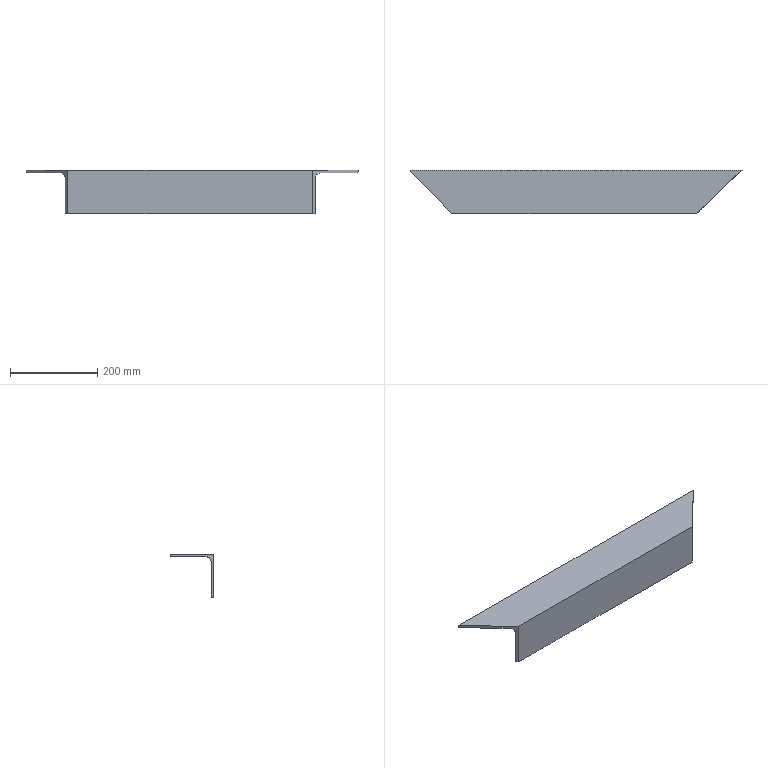Part | SolidWorks | features Extrusion 1, ICE 1 | 1 solid | 11 faces | box 761.728 x 100 x 100 mm | volume 732885 mm3 | plane 8 | cylinder 3 | commonest cylinder face diameters 5.4 x2 24 x1
STEP:
#1=CARTESIAN_POINT('',(-821.429,-32.,44.));
#2=VERTEX_POINT('',#1);
#3=CARTESIAN_POINT('',(-809.931,-44.,32.));
#4=VERTEX_POINT('',#3);
#5=CARTESIAN_POINT('',(-821.429,-32.,44.));
#6=CARTESIAN_POINT('',(-814.694,-39.029,44.));
#7=CARTESIAN_POINT('',(-809.931,-44.,39.029));
#8=CARTESIAN_POINT('',(-809.931,-44.,32.));
#9=(BOUNDED_CURVE()B_SPLINE_CURVE(3,(#5,#6,#7,#8),.UNSPECIFIED.,.F.,.F.)B_SPLINE_CURVE_WITH_KNOTS((4,4),(1.571,3.142),.UNSPECIFIED.)CURVE()GEOMETRIC_REPRESENTATION_ITEM()RATIONAL_B_SPLINE_CURVE((1.,0.8047,0.8047,1.))REPRESENTATION_ITEM(''));
#10=EDGE_CURVE('',#2,#4,#9,.T.);
#11=ORIENTED_EDGE('',*,*,#10,.F.);
#12=CARTESIAN_POINT('',(-223.851,-32.,44.));
#13=VERTEX_POINT('',#12);
#14=CARTESIAN_POINT('',(900.,-32.,44.));
#15=DIRECTION('',(-1.,0.,0.));
#16=VECTOR('',#15,1000.);
#17=LINE('',#14,#16);
#18=EDGE_CURVE('',#13,#2,#17,.T.);
#19=ORIENTED_EDGE('',*,*,#18,.F.);
#20=CARTESIAN_POINT('',(-236.375,-44.,32.));
#21=VERTEX_POINT('',#20);
#22=CARTESIAN_POINT('',(-236.375,-44.,32.));
#23=CARTESIAN_POINT('',(-236.375,-44.,39.029));
#24=CARTESIAN_POINT('',(-231.187,-39.029,44.));
#25=CARTESIAN_POINT('',(-223.851,-32.,44.));
#26=(BOUNDED_CURVE()B_SPLINE_CURVE(3,(#22,#23,#24,#25),.UNSPECIFIED.,.F.,.F.)B_SPLINE_CURVE_WITH_KNOTS((4,4),(0.,1.571),.UNSPECIFIED.)CURVE()GEOMETRIC_REPRESENTATION_ITEM()RATIONAL_B_SPLINE_CURVE((1.,0.8047,0.8047,1.))REPRESENTATION_ITEM(''));
#27=EDGE_CURVE('',#21,#13,#26,.T.);
#28=ORIENTED_EDGE('',*,*,#27,.F.);
#29=CARTESIAN_POINT('',(900.,-44.,32.));
#30=DIRECTION('',(-1.,0.,0.));
#31=VECTOR('',#30,1000.);
#32=LINE('',#29,#31);
#33=EDGE_CURVE('',#21,#4,#32,.T.);
#34=ORIENTED_EDGE('',*,*,#33,.T.);
#35=EDGE_LOOP('',(#11,#19,#28,#34));
#36=FACE_OUTER_BOUND('',#35,.T.);
#37=CARTESIAN_POINT('',(900.,-32.,32.));
#38=DIRECTION('',(-1.,0.,0.));
#39=DIRECTION('',(0.,0.,1.));
#40=AXIS2_PLACEMENT_3D('',#37,#38,#39);
#41=CYLINDRICAL_SURFACE('',#40,12.);
#42=ADVANCED_FACE('',(#36),#41,.F.);
#43=CARTESIAN_POINT('',(-897.413,47.3,44.));
#44=VERTEX_POINT('',#43);
#45=CARTESIAN_POINT('',(-37.074,-850.587,44.));
#46=DIRECTION('',(0.6918,-0.722,0.));
#47=VECTOR('',#46,1000.);
#48=LINE('',#45,#47);
#49=EDGE_CURVE('',#44,#2,#48,.T.);
#50=ORIENTED_EDGE('',*,*,#49,.F.);
#51=CARTESIAN_POINT('',(-141.09,47.3,44.));
#52=VERTEX_POINT('',#51);
#53=CARTESIAN_POINT('',(900.,47.3,44.));
#54=DIRECTION('',(-1.,0.,0.));
#55=VECTOR('',#54,1000.);
#56=LINE('',#53,#55);
#57=EDGE_CURVE('',#52,#44,#56,.T.);
#58=ORIENTED_EDGE('',*,*,#57,.F.);
#59=CARTESIAN_POINT('',(401.678,567.371,44.));
#60=DIRECTION('',(0.722,0.6918,0.));
#61=VECTOR('',#60,1000.);
#62=LINE('',#59,#61);
#63=EDGE_CURVE('',#13,#52,#62,.T.);
#64=ORIENTED_EDGE('',*,*,#63,.F.);
#65=ORIENTED_EDGE('',*,*,#18,.T.);
#66=EDGE_LOOP('',(#50,#58,#64,#65));
#67=FACE_OUTER_BOUND('',#66,.T.);
#68=CARTESIAN_POINT('',(900.,47.3,44.));
#69=DIRECTION('',(0.,0.,1.));
#70=DIRECTION('',(0.,-1.,0.));
#71=AXIS2_PLACEMENT_3D('',#68,#69,#70);
#72=PLANE('',#71);
#73=ADVANCED_FACE('',(#67),#72,.F.);
#74=CARTESIAN_POINT('',(-900.,50.,46.7));
#75=VERTEX_POINT('',#74);
#76=CARTESIAN_POINT('',(-900.,50.,46.7));
#77=CARTESIAN_POINT('',(-900.,50.,45.118));
#78=CARTESIAN_POINT('',(-898.928,48.882,44.));
#79=CARTESIAN_POINT('',(-897.413,47.3,44.));
#80=(BOUNDED_CURVE()B_SPLINE_CURVE(3,(#76,#77,#78,#79),.UNSPECIFIED.,.F.,.F.)B_SPLINE_CURVE_WITH_KNOTS((4,4),(0.,1.571),.UNSPECIFIED.)CURVE()GEOMETRIC_REPRESENTATION_ITEM()RATIONAL_B_SPLINE_CURVE((1.,0.8047,0.8047,1.))REPRESENTATION_ITEM(''));
#81=EDGE_CURVE('',#75,#44,#80,.T.);
#82=ORIENTED_EDGE('',*,*,#81,.F.);
#83=CARTESIAN_POINT('',(-138.272,50.,46.7));
#84=VERTEX_POINT('',#83);
#85=CARTESIAN_POINT('',(900.,50.,46.7));
#86=DIRECTION('',(-1.,0.,0.));
#87=VECTOR('',#86,1000.);
#88=LINE('',#85,#87);
#89=EDGE_CURVE('',#84,#75,#88,.T.);
#90=ORIENTED_EDGE('',*,*,#89,.F.);
#91=CARTESIAN_POINT('',(-141.09,47.3,44.));
#92=CARTESIAN_POINT('',(-139.44,48.882,44.));
#93=CARTESIAN_POINT('',(-138.272,50.,45.118));
#94=CARTESIAN_POINT('',(-138.272,50.,46.7));
#95=(BOUNDED_CURVE()B_SPLINE_CURVE(3,(#91,#92,#93,#94),.UNSPECIFIED.,.F.,.F.)B_SPLINE_CURVE_WITH_KNOTS((4,4),(1.571,3.142),.UNSPECIFIED.)CURVE()GEOMETRIC_REPRESENTATION_ITEM()RATIONAL_B_SPLINE_CURVE((1.,0.8047,0.8047,1.))REPRESENTATION_ITEM(''));
#96=EDGE_CURVE('',#52,#84,#95,.T.);
#97=ORIENTED_EDGE('',*,*,#96,.F.);
#98=ORIENTED_EDGE('',*,*,#57,.T.);
#99=EDGE_LOOP('',(#82,#90,#97,#98));
#100=FACE_OUTER_BOUND('',#99,.T.);
#101=CARTESIAN_POINT('',(900.,47.3,46.7));
#102=DIRECTION('',(-1.,0.,0.));
#103=DIRECTION('',(0.,0.,1.));
#104=AXIS2_PLACEMENT_3D('',#101,#102,#103);
#105=CYLINDRICAL_SURFACE('',#104,2.7);
#106=ADVANCED_FACE('',(#100),#105,.T.);
#107=CARTESIAN_POINT('',(-138.272,50.,50.));
#108=VERTEX_POINT('',#107);
#109=CARTESIAN_POINT('',(-138.272,50.,-50.));
#110=DIRECTION('',(0.,0.,1.));
#111=VECTOR('',#110,1000.);
#112=LINE('',#109,#111);
#113=EDGE_CURVE('',#84,#108,#112,.T.);
#114=ORIENTED_EDGE('',*,*,#113,.F.);
#115=ORIENTED_EDGE('',*,*,#89,.T.);
#116=CARTESIAN_POINT('',(-900.,50.,50.));
#117=VERTEX_POINT('',#116);
#118=CARTESIAN_POINT('',(-900.,50.,50.));
#119=DIRECTION('',(0.,0.,1.));
#120=VECTOR('',#119,1000.);
#121=LINE('',#118,#120);
#122=EDGE_CURVE('',#75,#117,#121,.T.);
#123=ORIENTED_EDGE('',*,*,#122,.T.);
#124=CARTESIAN_POINT('',(900.,50.,50.));
#125=DIRECTION('',(-1.,0.,0.));
#126=VECTOR('',#125,1000.);
#127=LINE('',#124,#126);
#128=EDGE_CURVE('',#108,#117,#127,.T.);
#129=ORIENTED_EDGE('',*,*,#128,.F.);
#130=EDGE_LOOP('',(#114,#115,#123,#129));
#131=FACE_OUTER_BOUND('',#130,.T.);
#132=CARTESIAN_POINT('',(900.,50.,50.));
#133=DIRECTION('',(0.,-1.,0.));
#134=DIRECTION('',(0.,0.,-1.));
#135=AXIS2_PLACEMENT_3D('',#132,#133,#134);
#136=PLANE('',#135);
#137=ADVANCED_FACE('',(#131),#136,.F.);
#138=CARTESIAN_POINT('',(-804.182,-50.,50.));
#139=VERTEX_POINT('',#138);
#140=CARTESIAN_POINT('',(-900.,50.,50.));
#141=DIRECTION('',(0.6918,-0.722,0.));
#142=VECTOR('',#141,1000.);
#143=LINE('',#140,#142);
#144=EDGE_CURVE('',#117,#139,#143,.T.);
#145=ORIENTED_EDGE('',*,*,#144,.T.);
#146=CARTESIAN_POINT('',(-242.637,-50.,50.));
#147=VERTEX_POINT('',#146);
#148=CARTESIAN_POINT('',(900.,-50.,50.));
#149=DIRECTION('',(-1.,0.,0.));
#150=VECTOR('',#149,1000.);
#151=LINE('',#148,#150);
#152=EDGE_CURVE('',#147,#139,#151,.T.);
#153=ORIENTED_EDGE('',*,*,#152,.F.);
#154=CARTESIAN_POINT('',(-535.396,-330.517,50.));
#155=DIRECTION('',(0.722,0.6918,0.));
#156=VECTOR('',#155,1000.);
#157=LINE('',#154,#156);
#158=EDGE_CURVE('',#147,#108,#157,.T.);
#159=ORIENTED_EDGE('',*,*,#158,.T.);
#160=ORIENTED_EDGE('',*,*,#128,.T.);
#161=EDGE_LOOP('',(#145,#153,#159,#160));
#162=FACE_OUTER_BOUND('',#161,.T.);
#163=CARTESIAN_POINT('',(900.,-50.,50.));
#164=DIRECTION('',(0.,0.,-1.));
#165=DIRECTION('',(0.,1.,0.));
#166=AXIS2_PLACEMENT_3D('',#163,#164,#165);
#167=PLANE('',#166);
#168=ADVANCED_FACE('',(#162),#167,.F.);
#169=CARTESIAN_POINT('',(-804.182,-50.,-50.));
#170=VERTEX_POINT('',#169);
#171=CARTESIAN_POINT('',(-804.182,-50.,-50.));
#172=DIRECTION('',(0.,0.,1.));
#173=VECTOR('',#172,1000.);
#174=LINE('',#171,#173);
#175=EDGE_CURVE('',#170,#139,#174,.T.);
#176=ORIENTED_EDGE('',*,*,#175,.F.);
#177=CARTESIAN_POINT('',(-242.637,-50.,-50.));
#178=VERTEX_POINT('',#177);
#179=CARTESIAN_POINT('',(900.,-50.,-50.));
#180=DIRECTION('',(-1.,0.,0.));
#181=VECTOR('',#180,1000.);
#182=LINE('',#179,#181);
#183=EDGE_CURVE('',#178,#170,#182,.T.);
#184=ORIENTED_EDGE('',*,*,#183,.F.);
#185=CARTESIAN_POINT('',(-242.637,-50.,-50.));
#186=DIRECTION('',(0.,0.,-1.));
#187=VECTOR('',#186,1000.);
#188=LINE('',#185,#187);
#189=EDGE_CURVE('',#147,#178,#188,.T.);
#190=ORIENTED_EDGE('',*,*,#189,.F.);
#191=ORIENTED_EDGE('',*,*,#152,.T.);
#192=EDGE_LOOP('',(#176,#184,#190,#191));
#193=FACE_OUTER_BOUND('',#192,.T.);
#194=CARTESIAN_POINT('',(900.,-50.,-50.));
#195=DIRECTION('',(0.,1.,0.));
#196=DIRECTION('',(0.,0.,1.));
#197=AXIS2_PLACEMENT_3D('',#194,#195,#196);
#198=PLANE('',#197);
#199=ADVANCED_FACE('',(#193),#198,.F.);
#200=CARTESIAN_POINT('',(-807.344,-46.7,-50.));
#201=VERTEX_POINT('',#200);
#202=CARTESIAN_POINT('',(-900.,50.,-50.));
#203=DIRECTION('',(0.6918,-0.722,0.));
#204=VECTOR('',#203,1000.);
#205=LINE('',#202,#204);
#206=EDGE_CURVE('',#201,#170,#205,.T.);
#207=ORIENTED_EDGE('',*,*,#206,.F.);
#208=CARTESIAN_POINT('',(-239.193,-46.7,-50.));
#209=VERTEX_POINT('',#208);
#210=CARTESIAN_POINT('',(900.,-46.7,-50.));
#211=DIRECTION('',(-1.,0.,0.));
#212=VECTOR('',#211,1000.);
#213=LINE('',#210,#212);
#214=EDGE_CURVE('',#209,#201,#213,.T.);
#215=ORIENTED_EDGE('',*,*,#214,.F.);
#216=CARTESIAN_POINT('',(-535.396,-330.517,-50.));
#217=DIRECTION('',(0.722,0.6918,0.));
#218=VECTOR('',#217,1000.);
#219=LINE('',#216,#218);
#220=EDGE_CURVE('',#178,#209,#219,.T.);
#221=ORIENTED_EDGE('',*,*,#220,.F.);
#222=ORIENTED_EDGE('',*,*,#183,.T.);
#223=EDGE_LOOP('',(#207,#215,#221,#222));
#224=FACE_OUTER_BOUND('',#223,.T.);
#225=CARTESIAN_POINT('',(900.,-46.7,-50.));
#226=DIRECTION('',(0.,0.,1.));
#227=DIRECTION('',(1.,0.,0.));
#228=AXIS2_PLACEMENT_3D('',#225,#226,#227);
#229=PLANE('',#228);
#230=ADVANCED_FACE('',(#224),#229,.F.);
#231=CARTESIAN_POINT('',(-809.931,-44.,-47.3));
#232=VERTEX_POINT('',#231);
#233=CARTESIAN_POINT('',(-809.931,-44.,-47.3));
#234=CARTESIAN_POINT('',(-809.931,-44.,-48.882));
#235=CARTESIAN_POINT('',(-808.859,-45.118,-50.));
#236=CARTESIAN_POINT('',(-807.344,-46.7,-50.));
#237=(BOUNDED_CURVE()B_SPLINE_CURVE(3,(#233,#234,#235,#236),.UNSPECIFIED.,.F.,.F.)B_SPLINE_CURVE_WITH_KNOTS((4,4),(0.,1.571),.UNSPECIFIED.)CURVE()GEOMETRIC_REPRESENTATION_ITEM()RATIONAL_B_SPLINE_CURVE((1.,0.8047,0.8047,1.))REPRESENTATION_ITEM(''));
#238=EDGE_CURVE('',#232,#201,#237,.T.);
#239=ORIENTED_EDGE('',*,*,#238,.F.);
#240=CARTESIAN_POINT('',(-236.375,-44.,-47.3));
#241=VERTEX_POINT('',#240);
#242=CARTESIAN_POINT('',(900.,-44.,-47.3));
#243=DIRECTION('',(-1.,0.,0.));
#244=VECTOR('',#243,1000.);
#245=LINE('',#242,#244);
#246=EDGE_CURVE('',#241,#232,#245,.T.);
#247=ORIENTED_EDGE('',*,*,#246,.F.);
#248=CARTESIAN_POINT('',(-239.193,-46.7,-50.));
#249=CARTESIAN_POINT('',(-237.542,-45.118,-50.));
#250=CARTESIAN_POINT('',(-236.375,-44.,-48.882));
#251=CARTESIAN_POINT('',(-236.375,-44.,-47.3));
#252=(BOUNDED_CURVE()B_SPLINE_CURVE(3,(#248,#249,#250,#251),.UNSPECIFIED.,.F.,.T.)B_SPLINE_CURVE_WITH_KNOTS((4,4),(1.571,3.142),.UNSPECIFIED.)CURVE()GEOMETRIC_REPRESENTATION_ITEM()RATIONAL_B_SPLINE_CURVE((1.,0.8047,0.8047,1.))REPRESENTATION_ITEM(''));
#253=EDGE_CURVE('',#209,#241,#252,.T.);
#254=ORIENTED_EDGE('',*,*,#253,.F.);
#255=ORIENTED_EDGE('',*,*,#214,.T.);
#256=EDGE_LOOP('',(#239,#247,#254,#255));
#257=FACE_OUTER_BOUND('',#256,.T.);
#258=CARTESIAN_POINT('',(900.,-46.7,-47.3));
#259=DIRECTION('',(-1.,0.,0.));
#260=DIRECTION('',(0.,0.,1.));
#261=AXIS2_PLACEMENT_3D('',#258,#259,#260);
#262=CYLINDRICAL_SURFACE('',#261,2.7);
#263=ADVANCED_FACE('',(#257),#262,.T.);
#264=CARTESIAN_POINT('',(-809.931,-44.,32.));
#265=DIRECTION('',(0.,0.,-1.));
#266=VECTOR('',#265,1000.);
#267=LINE('',#264,#266);
#268=EDGE_CURVE('',#4,#232,#267,.T.);
#269=ORIENTED_EDGE('',*,*,#268,.F.);
#270=ORIENTED_EDGE('',*,*,#33,.F.);
#271=CARTESIAN_POINT('',(-236.375,-44.,32.));
#272=DIRECTION('',(0.,0.,1.));
#273=VECTOR('',#272,1000.);
#274=LINE('',#271,#273);
#275=EDGE_CURVE('',#241,#21,#274,.T.);
#276=ORIENTED_EDGE('',*,*,#275,.F.);
#277=ORIENTED_EDGE('',*,*,#246,.T.);
#278=EDGE_LOOP('',(#269,#270,#276,#277));
#279=FACE_OUTER_BOUND('',#278,.T.);
#280=CARTESIAN_POINT('',(900.,-44.,32.));
#281=DIRECTION('',(0.,-1.,0.));
#282=DIRECTION('',(0.,0.,-1.));
#283=AXIS2_PLACEMENT_3D('',#280,#281,#282);
#284=PLANE('',#283);
#285=ADVANCED_FACE('',(#279),#284,.F.);
#286=ORIENTED_EDGE('',*,*,#175,.T.);
#287=ORIENTED_EDGE('',*,*,#144,.F.);
#288=ORIENTED_EDGE('',*,*,#122,.F.);
#289=ORIENTED_EDGE('',*,*,#81,.T.);
#290=ORIENTED_EDGE('',*,*,#49,.T.);
#291=ORIENTED_EDGE('',*,*,#10,.T.);
#292=ORIENTED_EDGE('',*,*,#268,.T.);
#293=ORIENTED_EDGE('',*,*,#238,.T.);
#294=ORIENTED_EDGE('',*,*,#206,.T.);
#295=EDGE_LOOP('',(#286,#287,#288,#289,#290,#291,#292,#293,#294));
#296=FACE_OUTER_BOUND('',#295,.T.);
#297=CARTESIAN_POINT('',(-900.,50.,-50.));
#298=DIRECTION('',(-0.722,-0.6918,0.));
#299=DIRECTION('',(0.6918,-0.722,0.));
#300=AXIS2_PLACEMENT_3D('',#297,#298,#299);
#301=PLANE('',#300);
#302=ADVANCED_FACE('',(#296),#301,.T.);
#303=ORIENTED_EDGE('',*,*,#189,.T.);
#304=ORIENTED_EDGE('',*,*,#220,.T.);
#305=ORIENTED_EDGE('',*,*,#253,.T.);
#306=ORIENTED_EDGE('',*,*,#275,.T.);
#307=ORIENTED_EDGE('',*,*,#27,.T.);
#308=ORIENTED_EDGE('',*,*,#63,.T.);
#309=ORIENTED_EDGE('',*,*,#96,.T.);
#310=ORIENTED_EDGE('',*,*,#113,.T.);
#311=ORIENTED_EDGE('',*,*,#158,.F.);
#312=EDGE_LOOP('',(#303,#304,#305,#306,#307,#308,#309,#310,#311));
#313=FACE_OUTER_BOUND('',#312,.T.);
#314=CARTESIAN_POINT('',(-535.396,-330.517,-50.));
#315=DIRECTION('',(0.6918,-0.722,0.));
#316=DIRECTION('',(0.722,0.6918,0.));
#317=AXIS2_PLACEMENT_3D('',#314,#315,#316);
#318=PLANE('',#317);
#319=ADVANCED_FACE('',(#313),#318,.T.);
#320=CLOSED_SHELL('',(#42,#73,#106,#137,#168,#199,#230,#263,#285,#302,#319));
#321=MANIFOLD_SOLID_BREP('',#320);
#322=CARTESIAN_POINT('',(0.,0.,0.));
#323=DIRECTION('',(0.,0.,1.));
#324=DIRECTION('',(1.,0.,0.));
#325=AXIS2_PLACEMENT_3D('',#322,#323,#324);
#326=(LENGTH_UNIT()NAMED_UNIT(*)SI_UNIT(.MILLI.,.METRE.));
#327=UNCERTAINTY_MEASURE_WITH_UNIT(LENGTH_MEASURE(0.00001),#326,'','');
#328=(NAMED_UNIT(*)PLANE_ANGLE_UNIT()SI_UNIT($,.RADIAN.));
#329=(NAMED_UNIT(*)SI_UNIT($,.STERADIAN.)SOLID_ANGLE_UNIT());
#330=(GEOMETRIC_REPRESENTATION_CONTEXT(3)GLOBAL_UNCERTAINTY_ASSIGNED_CONTEXT((#327))GLOBAL_UNIT_ASSIGNED_CONTEXT((#326,#328,#329))REPRESENTATION_CONTEXT('',''));
#331=ADVANCED_BREP_SHAPE_REPRESENTATION('',(#321,#325),#330);